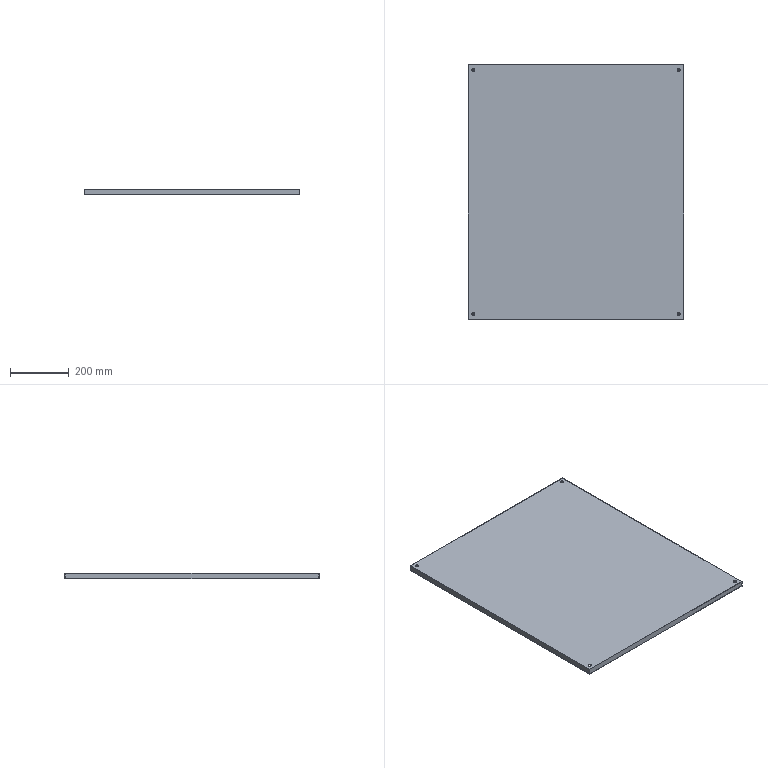Part | SolidWorks | features Extrusion 1, HoleWzd 1, ICE 1, Shell 1 | 1 solid | 32 faces | box 734 x 865.5 x 20 mm | volume 1496392 mm3 | cylinder 16 | plane 16 | commonest cylinder face diameters 6.6 x8 11 x8
STEP:
#1=CARTESIAN_POINT('',(-344.5,415.75,18.));
#2=VERTEX_POINT('',#1);
#3=CARTESIAN_POINT('',(-355.5,415.75,18.));
#4=VERTEX_POINT('',#3);
#5=CARTESIAN_POINT('',(-350.,415.75,18.));
#6=DIRECTION('',(0.,0.,-1.));
#7=DIRECTION('',(-1.,0.,0.));
#8=AXIS2_PLACEMENT_3D('',#5,#6,#7);
#9=CIRCLE('',#8,5.5);
#10=EDGE_CURVE('',#2,#4,#9,.T.);
#11=ORIENTED_EDGE('',*,*,#10,.T.);
#12=CARTESIAN_POINT('',(-355.5,415.75,20.));
#13=VERTEX_POINT('',#12);
#14=CARTESIAN_POINT('',(-355.5,415.75,20.));
#15=DIRECTION('',(0.,0.,1.));
#16=VECTOR('',#15,1000.);
#17=LINE('',#14,#16);
#18=EDGE_CURVE('',#4,#13,#17,.T.);
#19=ORIENTED_EDGE('',*,*,#18,.T.);
#20=CARTESIAN_POINT('',(-344.5,415.75,20.));
#21=VERTEX_POINT('',#20);
#22=CARTESIAN_POINT('',(-350.,415.75,20.));
#23=DIRECTION('',(0.,0.,1.));
#24=DIRECTION('',(1.,0.,0.));
#25=AXIS2_PLACEMENT_3D('',#22,#23,#24);
#26=CIRCLE('',#25,5.5);
#27=EDGE_CURVE('',#13,#21,#26,.T.);
#28=ORIENTED_EDGE('',*,*,#27,.T.);
#29=CARTESIAN_POINT('',(-344.5,415.75,20.));
#30=DIRECTION('',(0.,0.,1.));
#31=VECTOR('',#30,1000.);
#32=LINE('',#29,#31);
#33=EDGE_CURVE('',#2,#21,#32,.T.);
#34=ORIENTED_EDGE('',*,*,#33,.F.);
#35=EDGE_LOOP('',(#11,#19,#28,#34));
#36=FACE_OUTER_BOUND('',#35,.T.);
#37=CARTESIAN_POINT('',(-350.,415.75,20.));
#38=DIRECTION('',(0.,0.,1.));
#39=DIRECTION('',(1.,0.,0.));
#40=AXIS2_PLACEMENT_3D('',#37,#38,#39);
#41=CYLINDRICAL_SURFACE('',#40,5.5);
#42=ADVANCED_FACE('',(#36),#41,.F.);
#43=CARTESIAN_POINT('',(-353.3,415.75,0.));
#44=VERTEX_POINT('',#43);
#45=CARTESIAN_POINT('',(-346.7,415.75,0.));
#46=VERTEX_POINT('',#45);
#47=CARTESIAN_POINT('',(-350.,415.75,0.));
#48=DIRECTION('',(0.,0.,1.));
#49=DIRECTION('',(1.,0.,0.));
#50=AXIS2_PLACEMENT_3D('',#47,#48,#49);
#51=CIRCLE('',#50,3.3);
#52=EDGE_CURVE('',#44,#46,#51,.T.);
#53=ORIENTED_EDGE('',*,*,#52,.F.);
#54=CARTESIAN_POINT('',(-353.3,415.75,2.));
#55=VERTEX_POINT('',#54);
#56=CARTESIAN_POINT('',(-353.3,415.75,20.));
#57=DIRECTION('',(0.,0.,1.));
#58=VECTOR('',#57,1000.);
#59=LINE('',#56,#58);
#60=EDGE_CURVE('',#44,#55,#59,.T.);
#61=ORIENTED_EDGE('',*,*,#60,.T.);
#62=CARTESIAN_POINT('',(-346.7,415.75,2.));
#63=VERTEX_POINT('',#62);
#64=CARTESIAN_POINT('',(-350.,415.75,2.));
#65=DIRECTION('',(0.,0.,-1.));
#66=DIRECTION('',(-1.,0.,0.));
#67=AXIS2_PLACEMENT_3D('',#64,#65,#66);
#68=CIRCLE('',#67,3.3);
#69=EDGE_CURVE('',#63,#55,#68,.T.);
#70=ORIENTED_EDGE('',*,*,#69,.F.);
#71=CARTESIAN_POINT('',(-346.7,415.75,20.));
#72=DIRECTION('',(0.,0.,1.));
#73=VECTOR('',#72,1000.);
#74=LINE('',#71,#73);
#75=EDGE_CURVE('',#46,#63,#74,.T.);
#76=ORIENTED_EDGE('',*,*,#75,.F.);
#77=EDGE_LOOP('',(#53,#61,#70,#76));
#78=FACE_OUTER_BOUND('',#77,.T.);
#79=CARTESIAN_POINT('',(-350.,415.75,20.));
#80=DIRECTION('',(0.,0.,1.));
#81=DIRECTION('',(1.,0.,0.));
#82=AXIS2_PLACEMENT_3D('',#79,#80,#81);
#83=CYLINDRICAL_SURFACE('',#82,3.3);
#84=ADVANCED_FACE('',(#78),#83,.F.);
#85=CARTESIAN_POINT('',(-344.5,-415.75,18.));
#86=VERTEX_POINT('',#85);
#87=CARTESIAN_POINT('',(-355.5,-415.75,18.));
#88=VERTEX_POINT('',#87);
#89=CARTESIAN_POINT('',(-350.,-415.75,18.));
#90=DIRECTION('',(0.,0.,-1.));
#91=DIRECTION('',(-1.,0.,0.));
#92=AXIS2_PLACEMENT_3D('',#89,#90,#91);
#93=CIRCLE('',#92,5.5);
#94=EDGE_CURVE('',#86,#88,#93,.T.);
#95=ORIENTED_EDGE('',*,*,#94,.T.);
#96=CARTESIAN_POINT('',(-355.5,-415.75,20.));
#97=VERTEX_POINT('',#96);
#98=CARTESIAN_POINT('',(-355.5,-415.75,20.));
#99=DIRECTION('',(0.,0.,1.));
#100=VECTOR('',#99,1000.);
#101=LINE('',#98,#100);
#102=EDGE_CURVE('',#88,#97,#101,.T.);
#103=ORIENTED_EDGE('',*,*,#102,.T.);
#104=CARTESIAN_POINT('',(-344.5,-415.75,20.));
#105=VERTEX_POINT('',#104);
#106=CARTESIAN_POINT('',(-350.,-415.75,20.));
#107=DIRECTION('',(0.,0.,1.));
#108=DIRECTION('',(1.,0.,0.));
#109=AXIS2_PLACEMENT_3D('',#106,#107,#108);
#110=CIRCLE('',#109,5.5);
#111=EDGE_CURVE('',#97,#105,#110,.T.);
#112=ORIENTED_EDGE('',*,*,#111,.T.);
#113=CARTESIAN_POINT('',(-344.5,-415.75,20.));
#114=DIRECTION('',(0.,0.,1.));
#115=VECTOR('',#114,1000.);
#116=LINE('',#113,#115);
#117=EDGE_CURVE('',#86,#105,#116,.T.);
#118=ORIENTED_EDGE('',*,*,#117,.F.);
#119=EDGE_LOOP('',(#95,#103,#112,#118));
#120=FACE_OUTER_BOUND('',#119,.T.);
#121=CARTESIAN_POINT('',(-350.,-415.75,20.));
#122=DIRECTION('',(0.,0.,1.));
#123=DIRECTION('',(1.,0.,0.));
#124=AXIS2_PLACEMENT_3D('',#121,#122,#123);
#125=CYLINDRICAL_SURFACE('',#124,5.5);
#126=ADVANCED_FACE('',(#120),#125,.F.);
#127=CARTESIAN_POINT('',(-353.3,-415.75,0.));
#128=VERTEX_POINT('',#127);
#129=CARTESIAN_POINT('',(-346.7,-415.75,0.));
#130=VERTEX_POINT('',#129);
#131=CARTESIAN_POINT('',(-350.,-415.75,0.));
#132=DIRECTION('',(0.,0.,1.));
#133=DIRECTION('',(1.,0.,0.));
#134=AXIS2_PLACEMENT_3D('',#131,#132,#133);
#135=CIRCLE('',#134,3.3);
#136=EDGE_CURVE('',#128,#130,#135,.T.);
#137=ORIENTED_EDGE('',*,*,#136,.F.);
#138=CARTESIAN_POINT('',(-353.3,-415.75,2.));
#139=VERTEX_POINT('',#138);
#140=CARTESIAN_POINT('',(-353.3,-415.75,20.));
#141=DIRECTION('',(0.,0.,1.));
#142=VECTOR('',#141,1000.);
#143=LINE('',#140,#142);
#144=EDGE_CURVE('',#128,#139,#143,.T.);
#145=ORIENTED_EDGE('',*,*,#144,.T.);
#146=CARTESIAN_POINT('',(-346.7,-415.75,2.));
#147=VERTEX_POINT('',#146);
#148=CARTESIAN_POINT('',(-350.,-415.75,2.));
#149=DIRECTION('',(0.,0.,-1.));
#150=DIRECTION('',(-1.,0.,0.));
#151=AXIS2_PLACEMENT_3D('',#148,#149,#150);
#152=CIRCLE('',#151,3.3);
#153=EDGE_CURVE('',#147,#139,#152,.T.);
#154=ORIENTED_EDGE('',*,*,#153,.F.);
#155=CARTESIAN_POINT('',(-346.7,-415.75,20.));
#156=DIRECTION('',(0.,0.,1.));
#157=VECTOR('',#156,1000.);
#158=LINE('',#155,#157);
#159=EDGE_CURVE('',#130,#147,#158,.T.);
#160=ORIENTED_EDGE('',*,*,#159,.F.);
#161=EDGE_LOOP('',(#137,#145,#154,#160));
#162=FACE_OUTER_BOUND('',#161,.T.);
#163=CARTESIAN_POINT('',(-350.,-415.75,20.));
#164=DIRECTION('',(0.,0.,1.));
#165=DIRECTION('',(1.,0.,0.));
#166=AXIS2_PLACEMENT_3D('',#163,#164,#165);
#167=CYLINDRICAL_SURFACE('',#166,3.3);
#168=ADVANCED_FACE('',(#162),#167,.F.);
#169=CARTESIAN_POINT('',(346.7,-415.75,0.));
#170=VERTEX_POINT('',#169);
#171=CARTESIAN_POINT('',(353.3,-415.75,0.));
#172=VERTEX_POINT('',#171);
#173=CARTESIAN_POINT('',(350.,-415.75,0.));
#174=DIRECTION('',(0.,0.,1.));
#175=DIRECTION('',(1.,0.,0.));
#176=AXIS2_PLACEMENT_3D('',#173,#174,#175);
#177=CIRCLE('',#176,3.3);
#178=EDGE_CURVE('',#170,#172,#177,.T.);
#179=ORIENTED_EDGE('',*,*,#178,.F.);
#180=CARTESIAN_POINT('',(346.7,-415.75,2.));
#181=VERTEX_POINT('',#180);
#182=CARTESIAN_POINT('',(346.7,-415.75,20.));
#183=DIRECTION('',(0.,0.,1.));
#184=VECTOR('',#183,1000.);
#185=LINE('',#182,#184);
#186=EDGE_CURVE('',#170,#181,#185,.T.);
#187=ORIENTED_EDGE('',*,*,#186,.T.);
#188=CARTESIAN_POINT('',(353.3,-415.75,2.));
#189=VERTEX_POINT('',#188);
#190=CARTESIAN_POINT('',(350.,-415.75,2.));
#191=DIRECTION('',(0.,0.,-1.));
#192=DIRECTION('',(-1.,0.,0.));
#193=AXIS2_PLACEMENT_3D('',#190,#191,#192);
#194=CIRCLE('',#193,3.3);
#195=EDGE_CURVE('',#189,#181,#194,.T.);
#196=ORIENTED_EDGE('',*,*,#195,.F.);
#197=CARTESIAN_POINT('',(353.3,-415.75,20.));
#198=DIRECTION('',(0.,0.,1.));
#199=VECTOR('',#198,1000.);
#200=LINE('',#197,#199);
#201=EDGE_CURVE('',#172,#189,#200,.T.);
#202=ORIENTED_EDGE('',*,*,#201,.F.);
#203=EDGE_LOOP('',(#179,#187,#196,#202));
#204=FACE_OUTER_BOUND('',#203,.T.);
#205=CARTESIAN_POINT('',(350.,-415.75,20.));
#206=DIRECTION('',(0.,0.,1.));
#207=DIRECTION('',(1.,0.,0.));
#208=AXIS2_PLACEMENT_3D('',#205,#206,#207);
#209=CYLINDRICAL_SURFACE('',#208,3.3);
#210=ADVANCED_FACE('',(#204),#209,.F.);
#211=CARTESIAN_POINT('',(355.5,-415.75,18.));
#212=VERTEX_POINT('',#211);
#213=CARTESIAN_POINT('',(344.5,-415.75,18.));
#214=VERTEX_POINT('',#213);
#215=CARTESIAN_POINT('',(350.,-415.75,18.));
#216=DIRECTION('',(0.,0.,-1.));
#217=DIRECTION('',(-1.,0.,0.));
#218=AXIS2_PLACEMENT_3D('',#215,#216,#217);
#219=CIRCLE('',#218,5.5);
#220=EDGE_CURVE('',#212,#214,#219,.T.);
#221=ORIENTED_EDGE('',*,*,#220,.T.);
#222=CARTESIAN_POINT('',(344.5,-415.75,20.));
#223=VERTEX_POINT('',#222);
#224=CARTESIAN_POINT('',(344.5,-415.75,20.));
#225=DIRECTION('',(0.,0.,1.));
#226=VECTOR('',#225,1000.);
#227=LINE('',#224,#226);
#228=EDGE_CURVE('',#214,#223,#227,.T.);
#229=ORIENTED_EDGE('',*,*,#228,.T.);
#230=CARTESIAN_POINT('',(355.5,-415.75,20.));
#231=VERTEX_POINT('',#230);
#232=CARTESIAN_POINT('',(350.,-415.75,20.));
#233=DIRECTION('',(0.,0.,1.));
#234=DIRECTION('',(1.,0.,0.));
#235=AXIS2_PLACEMENT_3D('',#232,#233,#234);
#236=CIRCLE('',#235,5.5);
#237=EDGE_CURVE('',#223,#231,#236,.T.);
#238=ORIENTED_EDGE('',*,*,#237,.T.);
#239=CARTESIAN_POINT('',(355.5,-415.75,20.));
#240=DIRECTION('',(0.,0.,1.));
#241=VECTOR('',#240,1000.);
#242=LINE('',#239,#241);
#243=EDGE_CURVE('',#212,#231,#242,.T.);
#244=ORIENTED_EDGE('',*,*,#243,.F.);
#245=EDGE_LOOP('',(#221,#229,#238,#244));
#246=FACE_OUTER_BOUND('',#245,.T.);
#247=CARTESIAN_POINT('',(350.,-415.75,20.));
#248=DIRECTION('',(0.,0.,1.));
#249=DIRECTION('',(1.,0.,0.));
#250=AXIS2_PLACEMENT_3D('',#247,#248,#249);
#251=CYLINDRICAL_SURFACE('',#250,5.5);
#252=ADVANCED_FACE('',(#246),#251,.F.);
#253=CARTESIAN_POINT('',(355.5,415.75,18.));
#254=VERTEX_POINT('',#253);
#255=CARTESIAN_POINT('',(344.5,415.75,18.));
#256=VERTEX_POINT('',#255);
#257=CARTESIAN_POINT('',(350.,415.75,18.));
#258=DIRECTION('',(0.,0.,-1.));
#259=DIRECTION('',(-1.,0.,0.));
#260=AXIS2_PLACEMENT_3D('',#257,#258,#259);
#261=CIRCLE('',#260,5.5);
#262=EDGE_CURVE('',#254,#256,#261,.T.);
#263=ORIENTED_EDGE('',*,*,#262,.T.);
#264=CARTESIAN_POINT('',(344.5,415.75,20.));
#265=VERTEX_POINT('',#264);
#266=CARTESIAN_POINT('',(344.5,415.75,20.));
#267=DIRECTION('',(0.,0.,1.));
#268=VECTOR('',#267,1000.);
#269=LINE('',#266,#268);
#270=EDGE_CURVE('',#256,#265,#269,.T.);
#271=ORIENTED_EDGE('',*,*,#270,.T.);
#272=CARTESIAN_POINT('',(355.5,415.75,20.));
#273=VERTEX_POINT('',#272);
#274=CARTESIAN_POINT('',(350.,415.75,20.));
#275=DIRECTION('',(0.,0.,1.));
#276=DIRECTION('',(1.,0.,0.));
#277=AXIS2_PLACEMENT_3D('',#274,#275,#276);
#278=CIRCLE('',#277,5.5);
#279=EDGE_CURVE('',#265,#273,#278,.T.);
#280=ORIENTED_EDGE('',*,*,#279,.T.);
#281=CARTESIAN_POINT('',(355.5,415.75,20.));
#282=DIRECTION('',(0.,0.,1.));
#283=VECTOR('',#282,1000.);
#284=LINE('',#281,#283);
#285=EDGE_CURVE('',#254,#273,#284,.T.);
#286=ORIENTED_EDGE('',*,*,#285,.F.);
#287=EDGE_LOOP('',(#263,#271,#280,#286));
#288=FACE_OUTER_BOUND('',#287,.T.);
#289=CARTESIAN_POINT('',(350.,415.75,20.));
#290=DIRECTION('',(0.,0.,1.));
#291=DIRECTION('',(1.,0.,0.));
#292=AXIS2_PLACEMENT_3D('',#289,#290,#291);
#293=CYLINDRICAL_SURFACE('',#292,5.5);
#294=ADVANCED_FACE('',(#288),#293,.F.);
#295=CARTESIAN_POINT('',(346.7,415.75,0.));
#296=VERTEX_POINT('',#295);
#297=CARTESIAN_POINT('',(353.3,415.75,0.));
#298=VERTEX_POINT('',#297);
#299=CARTESIAN_POINT('',(350.,415.75,0.));
#300=DIRECTION('',(0.,0.,1.));
#301=DIRECTION('',(1.,0.,0.));
#302=AXIS2_PLACEMENT_3D('',#299,#300,#301);
#303=CIRCLE('',#302,3.3);
#304=EDGE_CURVE('',#296,#298,#303,.T.);
#305=ORIENTED_EDGE('',*,*,#304,.F.);
#306=CARTESIAN_POINT('',(346.7,415.75,2.));
#307=VERTEX_POINT('',#306);
#308=CARTESIAN_POINT('',(346.7,415.75,20.));
#309=DIRECTION('',(0.,0.,1.));
#310=VECTOR('',#309,1000.);
#311=LINE('',#308,#310);
#312=EDGE_CURVE('',#296,#307,#311,.T.);
#313=ORIENTED_EDGE('',*,*,#312,.T.);
#314=CARTESIAN_POINT('',(353.3,415.75,2.));
#315=VERTEX_POINT('',#314);
#316=CARTESIAN_POINT('',(350.,415.75,2.));
#317=DIRECTION('',(0.,0.,-1.));
#318=DIRECTION('',(-1.,0.,0.));
#319=AXIS2_PLACEMENT_3D('',#316,#317,#318);
#320=CIRCLE('',#319,3.3);
#321=EDGE_CURVE('',#315,#307,#320,.T.);
#322=ORIENTED_EDGE('',*,*,#321,.F.);
#323=CARTESIAN_POINT('',(353.3,415.75,20.));
#324=DIRECTION('',(0.,0.,1.));
#325=VECTOR('',#324,1000.);
#326=LINE('',#323,#325);
#327=EDGE_CURVE('',#298,#315,#326,.T.);
#328=ORIENTED_EDGE('',*,*,#327,.F.);
#329=EDGE_LOOP('',(#305,#313,#322,#328));
#330=FACE_OUTER_BOUND('',#329,.T.);
#331=CARTESIAN_POINT('',(350.,415.75,20.));
#332=DIRECTION('',(0.,0.,1.));
#333=DIRECTION('',(1.,0.,0.));
#334=AXIS2_PLACEMENT_3D('',#331,#332,#333);
#335=CYLINDRICAL_SURFACE('',#334,3.3);
#336=ADVANCED_FACE('',(#330),#335,.F.);
#337=CARTESIAN_POINT('',(-350.,415.75,0.));
#338=DIRECTION('',(0.,0.,1.));
#339=DIRECTION('',(1.,0.,0.));
#340=AXIS2_PLACEMENT_3D('',#337,#338,#339);
#341=CIRCLE('',#340,3.3);
#342=EDGE_CURVE('',#46,#44,#341,.T.);
#343=ORIENTED_EDGE('',*,*,#342,.T.);
#344=ORIENTED_EDGE('',*,*,#52,.T.);
#345=EDGE_LOOP('',(#343,#344));
#346=FACE_BOUND('',#345,.T.);
#347=CARTESIAN_POINT('',(-350.,-415.75,0.));
#348=DIRECTION('',(0.,0.,1.));
#349=DIRECTION('',(1.,0.,0.));
#350=AXIS2_PLACEMENT_3D('',#347,#348,#349);
#351=CIRCLE('',#350,3.3);
#352=EDGE_CURVE('',#130,#128,#351,.T.);
#353=ORIENTED_EDGE('',*,*,#352,.T.);
#354=ORIENTED_EDGE('',*,*,#136,.T.);
#355=EDGE_LOOP('',(#353,#354));
#356=FACE_BOUND('',#355,.T.);
#357=CARTESIAN_POINT('',(350.,-415.75,0.));
#358=DIRECTION('',(0.,0.,1.));
#359=DIRECTION('',(1.,0.,0.));
#360=AXIS2_PLACEMENT_3D('',#357,#358,#359);
#361=CIRCLE('',#360,3.3);
#362=EDGE_CURVE('',#172,#170,#361,.T.);
#363=ORIENTED_EDGE('',*,*,#362,.T.);
#364=ORIENTED_EDGE('',*,*,#178,.T.);
#365=EDGE_LOOP('',(#363,#364));
#366=FACE_BOUND('',#365,.T.);
#367=CARTESIAN_POINT('',(350.,415.75,0.));
#368=DIRECTION('',(0.,0.,1.));
#369=DIRECTION('',(1.,0.,0.));
#370=AXIS2_PLACEMENT_3D('',#367,#368,#369);
#371=CIRCLE('',#370,3.3);
#372=EDGE_CURVE('',#298,#296,#371,.T.);
#373=ORIENTED_EDGE('',*,*,#372,.T.);
#374=ORIENTED_EDGE('',*,*,#304,.T.);
#375=EDGE_LOOP('',(#373,#374));
#376=FACE_BOUND('',#375,.T.);
#377=CARTESIAN_POINT('',(367.,-432.75,0.));
#378=VERTEX_POINT('',#377);
#379=CARTESIAN_POINT('',(367.,432.75,0.));
#380=VERTEX_POINT('',#379);
#381=CARTESIAN_POINT('',(367.,-432.75,0.));
#382=DIRECTION('',(0.,1.,0.));
#383=VECTOR('',#382,1000.);
#384=LINE('',#381,#383);
#385=EDGE_CURVE('',#378,#380,#384,.T.);
#386=ORIENTED_EDGE('',*,*,#385,.F.);
#387=CARTESIAN_POINT('',(-367.,-432.75,0.));
#388=VERTEX_POINT('',#387);
#389=CARTESIAN_POINT('',(-367.,-432.75,0.));
#390=DIRECTION('',(1.,0.,0.));
#391=VECTOR('',#390,1000.);
#392=LINE('',#389,#391);
#393=EDGE_CURVE('',#388,#378,#392,.T.);
#394=ORIENTED_EDGE('',*,*,#393,.F.);
#395=CARTESIAN_POINT('',(-367.,432.75,0.));
#396=VERTEX_POINT('',#395);
#397=CARTESIAN_POINT('',(-367.,-432.75,0.));
#398=DIRECTION('',(0.,-1.,0.));
#399=VECTOR('',#398,1000.);
#400=LINE('',#397,#399);
#401=EDGE_CURVE('',#396,#388,#400,.T.);
#402=ORIENTED_EDGE('',*,*,#401,.F.);
#403=CARTESIAN_POINT('',(-367.,432.75,0.));
#404=DIRECTION('',(-1.,0.,0.));
#405=VECTOR('',#404,1000.);
#406=LINE('',#403,#405);
#407=EDGE_CURVE('',#380,#396,#406,.T.);
#408=ORIENTED_EDGE('',*,*,#407,.F.);
#409=EDGE_LOOP('',(#386,#394,#402,#408));
#410=FACE_OUTER_BOUND('',#409,.T.);
#411=CARTESIAN_POINT('',(347.,-412.75,0.));
#412=VERTEX_POINT('',#411);
#413=CARTESIAN_POINT('',(-347.,-412.75,0.));
#414=VERTEX_POINT('',#413);
#415=CARTESIAN_POINT('',(347.,-412.75,0.));
#416=DIRECTION('',(-1.,0.,0.));
#417=VECTOR('',#416,1000.);
#418=LINE('',#415,#417);
#419=EDGE_CURVE('',#412,#414,#418,.T.);
#420=ORIENTED_EDGE('',*,*,#419,.F.);
#421=CARTESIAN_POINT('',(347.,412.75,0.));
#422=VERTEX_POINT('',#421);
#423=CARTESIAN_POINT('',(347.,-412.75,0.));
#424=DIRECTION('',(0.,1.,0.));
#425=VECTOR('',#424,1000.);
#426=LINE('',#423,#425);
#427=EDGE_CURVE('',#412,#422,#426,.T.);
#428=ORIENTED_EDGE('',*,*,#427,.T.);
#429=CARTESIAN_POINT('',(-347.,412.75,0.));
#430=VERTEX_POINT('',#429);
#431=CARTESIAN_POINT('',(347.,412.75,0.));
#432=DIRECTION('',(-1.,0.,0.));
#433=VECTOR('',#432,1000.);
#434=LINE('',#431,#433);
#435=EDGE_CURVE('',#422,#430,#434,.T.);
#436=ORIENTED_EDGE('',*,*,#435,.T.);
#437=CARTESIAN_POINT('',(-347.,-412.75,0.));
#438=DIRECTION('',(0.,1.,0.));
#439=VECTOR('',#438,1000.);
#440=LINE('',#437,#439);
#441=EDGE_CURVE('',#414,#430,#440,.T.);
#442=ORIENTED_EDGE('',*,*,#441,.F.);
#443=EDGE_LOOP('',(#420,#428,#436,#442));
#444=FACE_BOUND('',#443,.T.);
#445=CARTESIAN_POINT('',(0.,0.,0.));
#446=DIRECTION('',(0.,0.,-1.));
#447=DIRECTION('',(-1.,0.,0.));
#448=AXIS2_PLACEMENT_3D('',#445,#446,#447);
#449=PLANE('',#448);
#450=ADVANCED_FACE('',(#346,#356,#366,#376,#410,#444),#449,.T.);
#451=ORIENTED_EDGE('',*,*,#385,.T.);
#452=CARTESIAN_POINT('',(367.,432.75,20.));
#453=VERTEX_POINT('',#452);
#454=CARTESIAN_POINT('',(367.,432.75,20.));
#455=DIRECTION('',(0.,0.,-1.));
#456=VECTOR('',#455,1000.);
#457=LINE('',#454,#456);
#458=EDGE_CURVE('',#453,#380,#457,.T.);
#459=ORIENTED_EDGE('',*,*,#458,.F.);
#460=CARTESIAN_POINT('',(367.,-432.75,20.));
#461=VERTEX_POINT('',#460);
#462=CARTESIAN_POINT('',(367.,-432.75,20.));
#463=DIRECTION('',(0.,1.,0.));
#464=VECTOR('',#463,1000.);
#465=LINE('',#462,#464);
#466=EDGE_CURVE('',#461,#453,#465,.T.);
#467=ORIENTED_EDGE('',*,*,#466,.F.);
#468=CARTESIAN_POINT('',(367.,-432.75,20.));
#469=DIRECTION('',(0.,0.,-1.));
#470=VECTOR('',#469,1000.);
#471=LINE('',#468,#470);
#472=EDGE_CURVE('',#461,#378,#471,.T.);
#473=ORIENTED_EDGE('',*,*,#472,.T.);
#474=EDGE_LOOP('',(#451,#459,#467,#473));
#475=FACE_OUTER_BOUND('',#474,.T.);
#476=CARTESIAN_POINT('',(367.,-432.75,20.));
#477=DIRECTION('',(-1.,0.,0.));
#478=DIRECTION('',(0.,0.,1.));
#479=AXIS2_PLACEMENT_3D('',#476,#477,#478);
#480=PLANE('',#479);
#481=ADVANCED_FACE('',(#475),#480,.F.);
#482=ORIENTED_EDGE('',*,*,#407,.T.);
#483=CARTESIAN_POINT('',(-367.,432.75,20.));
#484=VERTEX_POINT('',#483);
#485=CARTESIAN_POINT('',(-367.,432.75,20.));
#486=DIRECTION('',(0.,0.,-1.));
#487=VECTOR('',#486,1000.);
#488=LINE('',#485,#487);
#489=EDGE_CURVE('',#484,#396,#488,.T.);
#490=ORIENTED_EDGE('',*,*,#489,.F.);
#491=CARTESIAN_POINT('',(-367.,432.75,20.));
#492=DIRECTION('',(-1.,0.,0.));
#493=VECTOR('',#492,1000.);
#494=LINE('',#491,#493);
#495=EDGE_CURVE('',#453,#484,#494,.T.);
#496=ORIENTED_EDGE('',*,*,#495,.F.);
#497=ORIENTED_EDGE('',*,*,#458,.T.);
#498=EDGE_LOOP('',(#482,#490,#496,#497));
#499=FACE_OUTER_BOUND('',#498,.T.);
#500=CARTESIAN_POINT('',(-367.,432.75,20.));
#501=DIRECTION('',(0.,-1.,0.));
#502=DIRECTION('',(0.,0.,-1.));
#503=AXIS2_PLACEMENT_3D('',#500,#501,#502);
#504=PLANE('',#503);
#505=ADVANCED_FACE('',(#499),#504,.F.);
#506=ORIENTED_EDGE('',*,*,#401,.T.);
#507=CARTESIAN_POINT('',(-367.,-432.75,20.));
#508=VERTEX_POINT('',#507);
#509=CARTESIAN_POINT('',(-367.,-432.75,20.));
#510=DIRECTION('',(0.,0.,-1.));
#511=VECTOR('',#510,1000.);
#512=LINE('',#509,#511);
#513=EDGE_CURVE('',#508,#388,#512,.T.);
#514=ORIENTED_EDGE('',*,*,#513,.F.);
#515=CARTESIAN_POINT('',(-367.,-432.75,20.));
#516=DIRECTION('',(0.,-1.,0.));
#517=VECTOR('',#516,1000.);
#518=LINE('',#515,#517);
#519=EDGE_CURVE('',#484,#508,#518,.T.);
#520=ORIENTED_EDGE('',*,*,#519,.F.);
#521=ORIENTED_EDGE('',*,*,#489,.T.);
#522=EDGE_LOOP('',(#506,#514,#520,#521));
#523=FACE_OUTER_BOUND('',#522,.T.);
#524=CARTESIAN_POINT('',(-367.,-432.75,20.));
#525=DIRECTION('',(1.,0.,0.));
#526=DIRECTION('',(0.,0.,-1.));
#527=AXIS2_PLACEMENT_3D('',#524,#525,#526);
#528=PLANE('',#527);
#529=ADVANCED_FACE('',(#523),#528,.F.);
#530=ORIENTED_EDGE('',*,*,#393,.T.);
#531=ORIENTED_EDGE('',*,*,#472,.F.);
#532=CARTESIAN_POINT('',(-367.,-432.75,20.));
#533=DIRECTION('',(1.,0.,0.));
#534=VECTOR('',#533,1000.);
#535=LINE('',#532,#534);
#536=EDGE_CURVE('',#508,#461,#535,.T.);
#537=ORIENTED_EDGE('',*,*,#536,.F.);
#538=ORIENTED_EDGE('',*,*,#513,.T.);
#539=EDGE_LOOP('',(#530,#531,#537,#538));
#540=FACE_OUTER_BOUND('',#539,.T.);
#541=CARTESIAN_POINT('',(-367.,-432.75,20.));
#542=DIRECTION('',(0.,1.,0.));
#543=DIRECTION('',(0.,0.,1.));
#544=AXIS2_PLACEMENT_3D('',#541,#542,#543);
#545=PLANE('',#544);
#546=ADVANCED_FACE('',(#540),#545,.F.);
#547=CARTESIAN_POINT('',(-350.,415.75,20.));
#548=DIRECTION('',(0.,0.,1.));
#549=DIRECTION('',(1.,0.,0.));
#550=AXIS2_PLACEMENT_3D('',#547,#548,#549);
#551=CIRCLE('',#550,5.5);
#552=EDGE_CURVE('',#21,#13,#551,.T.);
#553=ORIENTED_EDGE('',*,*,#552,.F.);
#554=ORIENTED_EDGE('',*,*,#27,.F.);
#555=EDGE_LOOP('',(#553,#554));
#556=FACE_BOUND('',#555,.T.);
#557=CARTESIAN_POINT('',(-350.,-415.75,20.));
#558=DIRECTION('',(0.,0.,1.));
#559=DIRECTION('',(1.,0.,0.));
#560=AXIS2_PLACEMENT_3D('',#557,#558,#559);
#561=CIRCLE('',#560,5.5);
#562=EDGE_CURVE('',#105,#97,#561,.T.);
#563=ORIENTED_EDGE('',*,*,#562,.F.);
#564=ORIENTED_EDGE('',*,*,#111,.F.);
#565=EDGE_LOOP('',(#563,#564));
#566=FACE_BOUND('',#565,.T.);
#567=CARTESIAN_POINT('',(350.,-415.75,20.));
#568=DIRECTION('',(0.,0.,1.));
#569=DIRECTION('',(1.,0.,0.));
#570=AXIS2_PLACEMENT_3D('',#567,#568,#569);
#571=CIRCLE('',#570,5.5);
#572=EDGE_CURVE('',#231,#223,#571,.T.);
#573=ORIENTED_EDGE('',*,*,#572,.F.);
#574=ORIENTED_EDGE('',*,*,#237,.F.);
#575=EDGE_LOOP('',(#573,#574));
#576=FACE_BOUND('',#575,.T.);
#577=CARTESIAN_POINT('',(350.,415.75,20.));
#578=DIRECTION('',(0.,0.,1.));
#579=DIRECTION('',(1.,0.,0.));
#580=AXIS2_PLACEMENT_3D('',#577,#578,#579);
#581=CIRCLE('',#580,5.5);
#582=EDGE_CURVE('',#273,#265,#581,.T.);
#583=ORIENTED_EDGE('',*,*,#582,.F.);
#584=ORIENTED_EDGE('',*,*,#279,.F.);
#585=EDGE_LOOP('',(#583,#584));
#586=FACE_BOUND('',#585,.T.);
#587=ORIENTED_EDGE('',*,*,#466,.T.);
#588=ORIENTED_EDGE('',*,*,#495,.T.);
#589=ORIENTED_EDGE('',*,*,#519,.T.);
#590=ORIENTED_EDGE('',*,*,#536,.T.);
#591=EDGE_LOOP('',(#587,#588,#589,#590));
#592=FACE_OUTER_BOUND('',#591,.T.);
#593=CARTESIAN_POINT('',(0.,0.,20.));
#594=DIRECTION('',(0.,0.,-1.));
#595=DIRECTION('',(-1.,0.,0.));
#596=AXIS2_PLACEMENT_3D('',#593,#594,#595);
#597=PLANE('',#596);
#598=ADVANCED_FACE('',(#556,#566,#576,#586,#592),#597,.F.);
#599=ORIENTED_EDGE('',*,*,#427,.F.);
#600=CARTESIAN_POINT('',(347.,-412.75,2.));
#601=VERTEX_POINT('',#600);
#602=CARTESIAN_POINT('',(347.,-412.75,2.));
#603=DIRECTION('',(0.,0.,-1.));
#604=VECTOR('',#603,1000.);
#605=LINE('',#602,#604);
#606=EDGE_CURVE('',#601,#412,#605,.T.);
#607=ORIENTED_EDGE('',*,*,#606,.F.);
#608=CARTESIAN_POINT('',(347.,412.75,2.));
#609=VERTEX_POINT('',#608);
#610=CARTESIAN_POINT('',(347.,-412.75,2.));
#611=DIRECTION('',(0.,1.,0.));
#612=VECTOR('',#611,1000.);
#613=LINE('',#610,#612);
#614=EDGE_CURVE('',#601,#609,#613,.T.);
#615=ORIENTED_EDGE('',*,*,#614,.T.);
#616=CARTESIAN_POINT('',(347.,412.75,2.));
#617=DIRECTION('',(0.,0.,-1.));
#618=VECTOR('',#617,1000.);
#619=LINE('',#616,#618);
#620=EDGE_CURVE('',#609,#422,#619,.T.);
#621=ORIENTED_EDGE('',*,*,#620,.T.);
#622=EDGE_LOOP('',(#599,#607,#615,#621));
#623=FACE_OUTER_BOUND('',#622,.T.);
#624=CARTESIAN_POINT('',(347.,-412.75,2.));
#625=DIRECTION('',(-1.,0.,0.));
#626=DIRECTION('',(0.,0.,1.));
#627=AXIS2_PLACEMENT_3D('',#624,#625,#626);
#628=PLANE('',#627);
#629=ADVANCED_FACE('',(#623),#628,.T.);
#630=ORIENTED_EDGE('',*,*,#435,.F.);
#631=ORIENTED_EDGE('',*,*,#620,.F.);
#632=CARTESIAN_POINT('',(-347.,412.75,2.));
#633=VERTEX_POINT('',#632);
#634=CARTESIAN_POINT('',(347.,412.75,2.));
#635=DIRECTION('',(-1.,0.,0.));
#636=VECTOR('',#635,1000.);
#637=LINE('',#634,#636);
#638=EDGE_CURVE('',#609,#633,#637,.T.);
#639=ORIENTED_EDGE('',*,*,#638,.T.);
#640=CARTESIAN_POINT('',(-347.,412.75,2.));
#641=DIRECTION('',(0.,0.,-1.));
#642=VECTOR('',#641,1000.);
#643=LINE('',#640,#642);
#644=EDGE_CURVE('',#633,#430,#643,.T.);
#645=ORIENTED_EDGE('',*,*,#644,.T.);
#646=EDGE_LOOP('',(#630,#631,#639,#645));
#647=FACE_OUTER_BOUND('',#646,.T.);
#648=CARTESIAN_POINT('',(347.,412.75,2.));
#649=DIRECTION('',(0.,-1.,0.));
#650=DIRECTION('',(0.,0.,-1.));
#651=AXIS2_PLACEMENT_3D('',#648,#649,#650);
#652=PLANE('',#651);
#653=ADVANCED_FACE('',(#647),#652,.T.);
#654=ORIENTED_EDGE('',*,*,#441,.T.);
#655=ORIENTED_EDGE('',*,*,#644,.F.);
#656=CARTESIAN_POINT('',(-347.,-412.75,2.));
#657=VERTEX_POINT('',#656);
#658=CARTESIAN_POINT('',(-347.,-412.75,2.));
#659=DIRECTION('',(0.,1.,0.));
#660=VECTOR('',#659,1000.);
#661=LINE('',#658,#660);
#662=EDGE_CURVE('',#657,#633,#661,.T.);
#663=ORIENTED_EDGE('',*,*,#662,.F.);
#664=CARTESIAN_POINT('',(-347.,-412.75,2.));
#665=DIRECTION('',(0.,0.,-1.));
#666=VECTOR('',#665,1000.);
#667=LINE('',#664,#666);
#668=EDGE_CURVE('',#657,#414,#667,.T.);
#669=ORIENTED_EDGE('',*,*,#668,.T.);
#670=EDGE_LOOP('',(#654,#655,#663,#669));
#671=FACE_OUTER_BOUND('',#670,.T.);
#672=CARTESIAN_POINT('',(-347.,-412.75,2.));
#673=DIRECTION('',(-1.,0.,0.));
#674=DIRECTION('',(0.,0.,1.));
#675=AXIS2_PLACEMENT_3D('',#672,#673,#674);
#676=PLANE('',#675);
#677=ADVANCED_FACE('',(#671),#676,.F.);
#678=ORIENTED_EDGE('',*,*,#419,.T.);
#679=ORIENTED_EDGE('',*,*,#668,.F.);
#680=CARTESIAN_POINT('',(347.,-412.75,2.));
#681=DIRECTION('',(-1.,0.,0.));
#682=VECTOR('',#681,1000.);
#683=LINE('',#680,#682);
#684=EDGE_CURVE('',#601,#657,#683,.T.);
#685=ORIENTED_EDGE('',*,*,#684,.F.);
#686=ORIENTED_EDGE('',*,*,#606,.T.);
#687=EDGE_LOOP('',(#678,#679,#685,#686));
#688=FACE_OUTER_BOUND('',#687,.T.);
#689=CARTESIAN_POINT('',(347.,-412.75,2.));
#690=DIRECTION('',(0.,-1.,0.));
#691=DIRECTION('',(0.,0.,-1.));
#692=AXIS2_PLACEMENT_3D('',#689,#690,#691);
#693=PLANE('',#692);
#694=ADVANCED_FACE('',(#688),#693,.F.);
#695=ORIENTED_EDGE('',*,*,#69,.T.);
#696=CARTESIAN_POINT('',(-350.,415.75,2.));
#697=DIRECTION('',(0.,0.,-1.));
#698=DIRECTION('',(-1.,0.,0.));
#699=AXIS2_PLACEMENT_3D('',#696,#697,#698);
#700=CIRCLE('',#699,3.3);
#701=EDGE_CURVE('',#55,#63,#700,.T.);
#702=ORIENTED_EDGE('',*,*,#701,.T.);
#703=EDGE_LOOP('',(#695,#702));
#704=FACE_BOUND('',#703,.T.);
#705=ORIENTED_EDGE('',*,*,#153,.T.);
#706=CARTESIAN_POINT('',(-350.,-415.75,2.));
#707=DIRECTION('',(0.,0.,-1.));
#708=DIRECTION('',(-1.,0.,0.));
#709=AXIS2_PLACEMENT_3D('',#706,#707,#708);
#710=CIRCLE('',#709,3.3);
#711=EDGE_CURVE('',#139,#147,#710,.T.);
#712=ORIENTED_EDGE('',*,*,#711,.T.);
#713=EDGE_LOOP('',(#705,#712));
#714=FACE_BOUND('',#713,.T.);
#715=ORIENTED_EDGE('',*,*,#195,.T.);
#716=CARTESIAN_POINT('',(350.,-415.75,2.));
#717=DIRECTION('',(0.,0.,-1.));
#718=DIRECTION('',(-1.,0.,0.));
#719=AXIS2_PLACEMENT_3D('',#716,#717,#718);
#720=CIRCLE('',#719,3.3);
#721=EDGE_CURVE('',#181,#189,#720,.T.);
#722=ORIENTED_EDGE('',*,*,#721,.T.);
#723=EDGE_LOOP('',(#715,#722));
#724=FACE_BOUND('',#723,.T.);
#725=ORIENTED_EDGE('',*,*,#321,.T.);
#726=CARTESIAN_POINT('',(350.,415.75,2.));
#727=DIRECTION('',(0.,0.,-1.));
#728=DIRECTION('',(-1.,0.,0.));
#729=AXIS2_PLACEMENT_3D('',#726,#727,#728);
#730=CIRCLE('',#729,3.3);
#731=EDGE_CURVE('',#307,#315,#730,.T.);
#732=ORIENTED_EDGE('',*,*,#731,.T.);
#733=EDGE_LOOP('',(#725,#732));
#734=FACE_BOUND('',#733,.T.);
#735=CARTESIAN_POINT('',(365.,-430.75,2.));
#736=VERTEX_POINT('',#735);
#737=CARTESIAN_POINT('',(365.,430.75,2.));
#738=VERTEX_POINT('',#737);
#739=CARTESIAN_POINT('',(365.,0.,2.));
#740=DIRECTION('',(0.,1.,0.));
#741=VECTOR('',#740,1000.);
#742=LINE('',#739,#741);
#743=EDGE_CURVE('',#736,#738,#742,.T.);
#744=ORIENTED_EDGE('',*,*,#743,.T.);
#745=CARTESIAN_POINT('',(-365.,430.75,2.));
#746=VERTEX_POINT('',#745);
#747=CARTESIAN_POINT('',(0.,430.75,2.));
#748=DIRECTION('',(-1.,0.,0.));
#749=VECTOR('',#748,1000.);
#750=LINE('',#747,#749);
#751=EDGE_CURVE('',#738,#746,#750,.T.);
#752=ORIENTED_EDGE('',*,*,#751,.T.);
#753=CARTESIAN_POINT('',(-365.,-430.75,2.));
#754=VERTEX_POINT('',#753);
#755=CARTESIAN_POINT('',(-365.,0.,2.));
#756=DIRECTION('',(0.,-1.,0.));
#757=VECTOR('',#756,1000.);
#758=LINE('',#755,#757);
#759=EDGE_CURVE('',#746,#754,#758,.T.);
#760=ORIENTED_EDGE('',*,*,#759,.T.);
#761=CARTESIAN_POINT('',(0.,-430.75,2.));
#762=DIRECTION('',(1.,0.,0.));
#763=VECTOR('',#762,1000.);
#764=LINE('',#761,#763);
#765=EDGE_CURVE('',#754,#736,#764,.T.);
#766=ORIENTED_EDGE('',*,*,#765,.T.);
#767=EDGE_LOOP('',(#744,#752,#760,#766));
#768=FACE_OUTER_BOUND('',#767,.T.);
#769=ORIENTED_EDGE('',*,*,#684,.T.);
#770=ORIENTED_EDGE('',*,*,#662,.T.);
#771=ORIENTED_EDGE('',*,*,#638,.F.);
#772=ORIENTED_EDGE('',*,*,#614,.F.);
#773=EDGE_LOOP('',(#769,#770,#771,#772));
#774=FACE_BOUND('',#773,.T.);
#775=CARTESIAN_POINT('',(0.,0.,2.));
#776=DIRECTION('',(0.,0.,-1.));
#777=DIRECTION('',(-1.,0.,0.));
#778=AXIS2_PLACEMENT_3D('',#775,#776,#777);
#779=PLANE('',#778);
#780=ADVANCED_FACE('',(#704,#714,#724,#734,#768,#774),#779,.F.);
#781=ORIENTED_EDGE('',*,*,#743,.F.);
#782=CARTESIAN_POINT('',(365.,-430.75,18.));
#783=VERTEX_POINT('',#782);
#784=CARTESIAN_POINT('',(365.,-430.75,20.));
#785=DIRECTION('',(0.,0.,-1.));
#786=VECTOR('',#785,1000.);
#787=LINE('',#784,#786);
#788=EDGE_CURVE('',#783,#736,#787,.T.);
#789=ORIENTED_EDGE('',*,*,#788,.F.);
#790=CARTESIAN_POINT('',(365.,430.75,18.));
#791=VERTEX_POINT('',#790);
#792=CARTESIAN_POINT('',(365.,0.,18.));
#793=DIRECTION('',(0.,1.,0.));
#794=VECTOR('',#793,1000.);
#795=LINE('',#792,#794);
#796=EDGE_CURVE('',#783,#791,#795,.T.);
#797=ORIENTED_EDGE('',*,*,#796,.T.);
#798=CARTESIAN_POINT('',(365.,430.75,20.));
#799=DIRECTION('',(0.,0.,-1.));
#800=VECTOR('',#799,1000.);
#801=LINE('',#798,#800);
#802=EDGE_CURVE('',#791,#738,#801,.T.);
#803=ORIENTED_EDGE('',*,*,#802,.T.);
#804=EDGE_LOOP('',(#781,#789,#797,#803));
#805=FACE_OUTER_BOUND('',#804,.T.);
#806=CARTESIAN_POINT('',(365.,-432.75,20.));
#807=DIRECTION('',(-1.,0.,0.));
#808=DIRECTION('',(0.,0.,1.));
#809=AXIS2_PLACEMENT_3D('',#806,#807,#808);
#810=PLANE('',#809);
#811=ADVANCED_FACE('',(#805),#810,.T.);
#812=ORIENTED_EDGE('',*,*,#751,.F.);
#813=ORIENTED_EDGE('',*,*,#802,.F.);
#814=CARTESIAN_POINT('',(-365.,430.75,18.));
#815=VERTEX_POINT('',#814);
#816=CARTESIAN_POINT('',(0.,430.75,18.));
#817=DIRECTION('',(-1.,0.,0.));
#818=VECTOR('',#817,1000.);
#819=LINE('',#816,#818);
#820=EDGE_CURVE('',#791,#815,#819,.T.);
#821=ORIENTED_EDGE('',*,*,#820,.T.);
#822=CARTESIAN_POINT('',(-365.,430.75,20.));
#823=DIRECTION('',(0.,0.,-1.));
#824=VECTOR('',#823,1000.);
#825=LINE('',#822,#824);
#826=EDGE_CURVE('',#815,#746,#825,.T.);
#827=ORIENTED_EDGE('',*,*,#826,.T.);
#828=EDGE_LOOP('',(#812,#813,#821,#827));
#829=FACE_OUTER_BOUND('',#828,.T.);
#830=CARTESIAN_POINT('',(-367.,430.75,20.));
#831=DIRECTION('',(0.,-1.,0.));
#832=DIRECTION('',(0.,0.,-1.));
#833=AXIS2_PLACEMENT_3D('',#830,#831,#832);
#834=PLANE('',#833);
#835=ADVANCED_FACE('',(#829),#834,.T.);
#836=ORIENTED_EDGE('',*,*,#759,.F.);
#837=ORIENTED_EDGE('',*,*,#826,.F.);
#838=CARTESIAN_POINT('',(-365.,-430.75,18.));
#839=VERTEX_POINT('',#838);
#840=CARTESIAN_POINT('',(-365.,0.,18.));
#841=DIRECTION('',(0.,-1.,0.));
#842=VECTOR('',#841,1000.);
#843=LINE('',#840,#842);
#844=EDGE_CURVE('',#815,#839,#843,.T.);
#845=ORIENTED_EDGE('',*,*,#844,.T.);
#846=CARTESIAN_POINT('',(-365.,-430.75,20.));
#847=DIRECTION('',(0.,0.,-1.));
#848=VECTOR('',#847,1000.);
#849=LINE('',#846,#848);
#850=EDGE_CURVE('',#839,#754,#849,.T.);
#851=ORIENTED_EDGE('',*,*,#850,.T.);
#852=EDGE_LOOP('',(#836,#837,#845,#851));
#853=FACE_OUTER_BOUND('',#852,.T.);
#854=CARTESIAN_POINT('',(-365.,-432.75,20.));
#855=DIRECTION('',(1.,0.,0.));
#856=DIRECTION('',(0.,0.,-1.));
#857=AXIS2_PLACEMENT_3D('',#854,#855,#856);
#858=PLANE('',#857);
#859=ADVANCED_FACE('',(#853),#858,.T.);
#860=ORIENTED_EDGE('',*,*,#765,.F.);
#861=ORIENTED_EDGE('',*,*,#850,.F.);
#862=CARTESIAN_POINT('',(0.,-430.75,18.));
#863=DIRECTION('',(1.,0.,0.));
#864=VECTOR('',#863,1000.);
#865=LINE('',#862,#864);
#866=EDGE_CURVE('',#839,#783,#865,.T.);
#867=ORIENTED_EDGE('',*,*,#866,.T.);
#868=ORIENTED_EDGE('',*,*,#788,.T.);
#869=EDGE_LOOP('',(#860,#861,#867,#868));
#870=FACE_OUTER_BOUND('',#869,.T.);
#871=CARTESIAN_POINT('',(-367.,-430.75,20.));
#872=DIRECTION('',(0.,1.,0.));
#873=DIRECTION('',(0.,0.,1.));
#874=AXIS2_PLACEMENT_3D('',#871,#872,#873);
#875=PLANE('',#874);
#876=ADVANCED_FACE('',(#870),#875,.T.);
#877=ORIENTED_EDGE('',*,*,#10,.F.);
#878=CARTESIAN_POINT('',(-350.,415.75,18.));
#879=DIRECTION('',(0.,0.,-1.));
#880=DIRECTION('',(-1.,0.,0.));
#881=AXIS2_PLACEMENT_3D('',#878,#879,#880);
#882=CIRCLE('',#881,5.5);
#883=EDGE_CURVE('',#4,#2,#882,.T.);
#884=ORIENTED_EDGE('',*,*,#883,.F.);
#885=EDGE_LOOP('',(#877,#884));
#886=FACE_BOUND('',#885,.T.);
#887=ORIENTED_EDGE('',*,*,#94,.F.);
#888=CARTESIAN_POINT('',(-350.,-415.75,18.));
#889=DIRECTION('',(0.,0.,-1.));
#890=DIRECTION('',(-1.,0.,0.));
#891=AXIS2_PLACEMENT_3D('',#888,#889,#890);
#892=CIRCLE('',#891,5.5);
#893=EDGE_CURVE('',#88,#86,#892,.T.);
#894=ORIENTED_EDGE('',*,*,#893,.F.);
#895=EDGE_LOOP('',(#887,#894));
#896=FACE_BOUND('',#895,.T.);
#897=ORIENTED_EDGE('',*,*,#220,.F.);
#898=CARTESIAN_POINT('',(350.,-415.75,18.));
#899=DIRECTION('',(0.,0.,-1.));
#900=DIRECTION('',(-1.,0.,0.));
#901=AXIS2_PLACEMENT_3D('',#898,#899,#900);
#902=CIRCLE('',#901,5.5);
#903=EDGE_CURVE('',#214,#212,#902,.T.);
#904=ORIENTED_EDGE('',*,*,#903,.F.);
#905=EDGE_LOOP('',(#897,#904));
#906=FACE_BOUND('',#905,.T.);
#907=ORIENTED_EDGE('',*,*,#262,.F.);
#908=CARTESIAN_POINT('',(350.,415.75,18.));
#909=DIRECTION('',(0.,0.,-1.));
#910=DIRECTION('',(-1.,0.,0.));
#911=AXIS2_PLACEMENT_3D('',#908,#909,#910);
#912=CIRCLE('',#911,5.5);
#913=EDGE_CURVE('',#256,#254,#912,.T.);
#914=ORIENTED_EDGE('',*,*,#913,.F.);
#915=EDGE_LOOP('',(#907,#914));
#916=FACE_BOUND('',#915,.T.);
#917=ORIENTED_EDGE('',*,*,#796,.F.);
#918=ORIENTED_EDGE('',*,*,#866,.F.);
#919=ORIENTED_EDGE('',*,*,#844,.F.);
#920=ORIENTED_EDGE('',*,*,#820,.F.);
#921=EDGE_LOOP('',(#917,#918,#919,#920));
#922=FACE_OUTER_BOUND('',#921,.T.);
#923=CARTESIAN_POINT('',(0.,0.,18.));
#924=DIRECTION('',(0.,0.,-1.));
#925=DIRECTION('',(-1.,0.,0.));
#926=AXIS2_PLACEMENT_3D('',#923,#924,#925);
#927=PLANE('',#926);
#928=ADVANCED_FACE('',(#886,#896,#906,#916,#922),#927,.T.);
#929=ORIENTED_EDGE('',*,*,#312,.F.);
#930=ORIENTED_EDGE('',*,*,#372,.F.);
#931=ORIENTED_EDGE('',*,*,#327,.T.);
#932=ORIENTED_EDGE('',*,*,#731,.F.);
#933=EDGE_LOOP('',(#929,#930,#931,#932));
#934=FACE_OUTER_BOUND('',#933,.T.);
#935=CARTESIAN_POINT('',(350.,415.75,20.));
#936=DIRECTION('',(0.,0.,1.));
#937=DIRECTION('',(1.,0.,0.));
#938=AXIS2_PLACEMENT_3D('',#935,#936,#937);
#939=CYLINDRICAL_SURFACE('',#938,3.3);
#940=ADVANCED_FACE('',(#934),#939,.F.);
#941=ORIENTED_EDGE('',*,*,#270,.F.);
#942=ORIENTED_EDGE('',*,*,#913,.T.);
#943=ORIENTED_EDGE('',*,*,#285,.T.);
#944=ORIENTED_EDGE('',*,*,#582,.T.);
#945=EDGE_LOOP('',(#941,#942,#943,#944));
#946=FACE_OUTER_BOUND('',#945,.T.);
#947=CARTESIAN_POINT('',(350.,415.75,20.));
#948=DIRECTION('',(0.,0.,1.));
#949=DIRECTION('',(1.,0.,0.));
#950=AXIS2_PLACEMENT_3D('',#947,#948,#949);
#951=CYLINDRICAL_SURFACE('',#950,5.5);
#952=ADVANCED_FACE('',(#946),#951,.F.);
#953=ORIENTED_EDGE('',*,*,#228,.F.);
#954=ORIENTED_EDGE('',*,*,#903,.T.);
#955=ORIENTED_EDGE('',*,*,#243,.T.);
#956=ORIENTED_EDGE('',*,*,#572,.T.);
#957=EDGE_LOOP('',(#953,#954,#955,#956));
#958=FACE_OUTER_BOUND('',#957,.T.);
#959=CARTESIAN_POINT('',(350.,-415.75,20.));
#960=DIRECTION('',(0.,0.,1.));
#961=DIRECTION('',(1.,0.,0.));
#962=AXIS2_PLACEMENT_3D('',#959,#960,#961);
#963=CYLINDRICAL_SURFACE('',#962,5.5);
#964=ADVANCED_FACE('',(#958),#963,.F.);
#965=ORIENTED_EDGE('',*,*,#186,.F.);
#966=ORIENTED_EDGE('',*,*,#362,.F.);
#967=ORIENTED_EDGE('',*,*,#201,.T.);
#968=ORIENTED_EDGE('',*,*,#721,.F.);
#969=EDGE_LOOP('',(#965,#966,#967,#968));
#970=FACE_OUTER_BOUND('',#969,.T.);
#971=CARTESIAN_POINT('',(350.,-415.75,20.));
#972=DIRECTION('',(0.,0.,1.));
#973=DIRECTION('',(1.,0.,0.));
#974=AXIS2_PLACEMENT_3D('',#971,#972,#973);
#975=CYLINDRICAL_SURFACE('',#974,3.3);
#976=ADVANCED_FACE('',(#970),#975,.F.);
#977=ORIENTED_EDGE('',*,*,#144,.F.);
#978=ORIENTED_EDGE('',*,*,#352,.F.);
#979=ORIENTED_EDGE('',*,*,#159,.T.);
#980=ORIENTED_EDGE('',*,*,#711,.F.);
#981=EDGE_LOOP('',(#977,#978,#979,#980));
#982=FACE_OUTER_BOUND('',#981,.T.);
#983=CARTESIAN_POINT('',(-350.,-415.75,20.));
#984=DIRECTION('',(0.,0.,1.));
#985=DIRECTION('',(1.,0.,0.));
#986=AXIS2_PLACEMENT_3D('',#983,#984,#985);
#987=CYLINDRICAL_SURFACE('',#986,3.3);
#988=ADVANCED_FACE('',(#982),#987,.F.);
#989=ORIENTED_EDGE('',*,*,#102,.F.);
#990=ORIENTED_EDGE('',*,*,#893,.T.);
#991=ORIENTED_EDGE('',*,*,#117,.T.);
#992=ORIENTED_EDGE('',*,*,#562,.T.);
#993=EDGE_LOOP('',(#989,#990,#991,#992));
#994=FACE_OUTER_BOUND('',#993,.T.);
#995=CARTESIAN_POINT('',(-350.,-415.75,20.));
#996=DIRECTION('',(0.,0.,1.));
#997=DIRECTION('',(1.,0.,0.));
#998=AXIS2_PLACEMENT_3D('',#995,#996,#997);
#999=CYLINDRICAL_SURFACE('',#998,5.5);
#1000=ADVANCED_FACE('',(#994),#999,.F.);
#1001=ORIENTED_EDGE('',*,*,#60,.F.);
#1002=ORIENTED_EDGE('',*,*,#342,.F.);
#1003=ORIENTED_EDGE('',*,*,#75,.T.);
#1004=ORIENTED_EDGE('',*,*,#701,.F.);
#1005=EDGE_LOOP('',(#1001,#1002,#1003,#1004));
#1006=FACE_OUTER_BOUND('',#1005,.T.);
#1007=CARTESIAN_POINT('',(-350.,415.75,20.));
#1008=DIRECTION('',(0.,0.,1.));
#1009=DIRECTION('',(1.,0.,0.));
#1010=AXIS2_PLACEMENT_3D('',#1007,#1008,#1009);
#1011=CYLINDRICAL_SURFACE('',#1010,3.3);
#1012=ADVANCED_FACE('',(#1006),#1011,.F.);
#1013=ORIENTED_EDGE('',*,*,#18,.F.);
#1014=ORIENTED_EDGE('',*,*,#883,.T.);
#1015=ORIENTED_EDGE('',*,*,#33,.T.);
#1016=ORIENTED_EDGE('',*,*,#552,.T.);
#1017=EDGE_LOOP('',(#1013,#1014,#1015,#1016));
#1018=FACE_OUTER_BOUND('',#1017,.T.);
#1019=CARTESIAN_POINT('',(-350.,415.75,20.));
#1020=DIRECTION('',(0.,0.,1.));
#1021=DIRECTION('',(1.,0.,0.));
#1022=AXIS2_PLACEMENT_3D('',#1019,#1020,#1021);
#1023=CYLINDRICAL_SURFACE('',#1022,5.5);
#1024=ADVANCED_FACE('',(#1018),#1023,.F.);
#1025=CLOSED_SHELL('',(#42,#84,#126,#168,#210,#252,#294,#336,#450,#481,#505,#529,#546,#598,#629,#653,#677,#694,#780,#811,#835,#859,#876,#928,#940,#952,#964,#976,#988,#1000,#1012,#1024));
#1026=MANIFOLD_SOLID_BREP('',#1025);
#1027=CARTESIAN_POINT('',(0.,0.,0.));
#1028=DIRECTION('',(0.,0.,1.));
#1029=DIRECTION('',(1.,0.,0.));
#1030=AXIS2_PLACEMENT_3D('',#1027,#1028,#1029);
#1031=(LENGTH_UNIT()NAMED_UNIT(*)SI_UNIT(.MILLI.,.METRE.));
#1032=UNCERTAINTY_MEASURE_WITH_UNIT(LENGTH_MEASURE(0.00001),#1031,'','');
#1033=(NAMED_UNIT(*)PLANE_ANGLE_UNIT()SI_UNIT($,.RADIAN.));
#1034=(NAMED_UNIT(*)SI_UNIT($,.STERADIAN.)SOLID_ANGLE_UNIT());
#1035=(GEOMETRIC_REPRESENTATION_CONTEXT(3)GLOBAL_UNCERTAINTY_ASSIGNED_CONTEXT((#1032))GLOBAL_UNIT_ASSIGNED_CONTEXT((#1031,#1033,#1034))REPRESENTATION_CONTEXT('',''));
#1036=ADVANCED_BREP_SHAPE_REPRESENTATION('',(#1026,#1030),#1035);